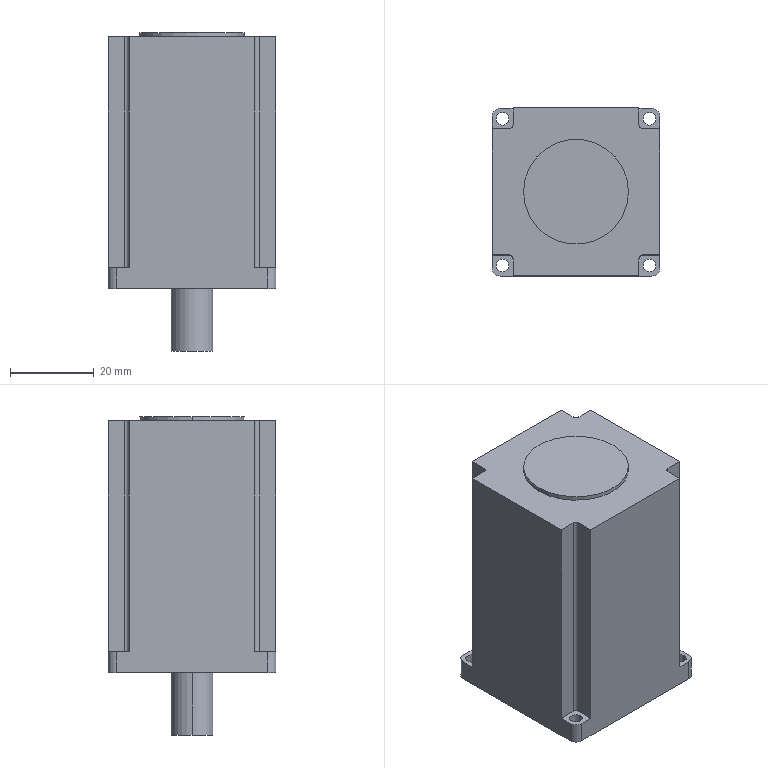Part | SolidWorks | features ICE 4, Fillet 2, Extrusion 1 | 1 solid | 40 faces | box 40 x 40 x 76 mm | volume 92058 mm3 | cylinder 20 | plane 20 | commonest cylinder face diameters 3 x8 2 x4 4 x4 10 x2 25 x2
STEP:
#1=CARTESIAN_POINT('',(-5.,0.,-45.));
#2=VERTEX_POINT('',#1);
#3=CARTESIAN_POINT('',(5.,0.,-45.));
#4=VERTEX_POINT('',#3);
#5=CARTESIAN_POINT('',(0.,0.,-45.));
#6=DIRECTION('',(0.,0.,-1.));
#7=DIRECTION('',(-1.,0.,0.));
#8=AXIS2_PLACEMENT_3D('',#5,#6,#7);
#9=CIRCLE('',#8,5.);
#10=EDGE_CURVE('',#2,#4,#9,.T.);
#11=ORIENTED_EDGE('',*,*,#10,.F.);
#12=CARTESIAN_POINT('',(-5.,0.,-30.));
#13=VERTEX_POINT('',#12);
#14=CARTESIAN_POINT('',(-5.,0.,-45.));
#15=DIRECTION('',(0.,0.,1.));
#16=VECTOR('',#15,1000.);
#17=LINE('',#14,#16);
#18=EDGE_CURVE('',#2,#13,#17,.T.);
#19=ORIENTED_EDGE('',*,*,#18,.T.);
#20=CARTESIAN_POINT('',(5.,0.,-30.));
#21=VERTEX_POINT('',#20);
#22=CARTESIAN_POINT('',(0.,0.,-30.));
#23=DIRECTION('',(0.,0.,-1.));
#24=DIRECTION('',(1.,0.,0.));
#25=AXIS2_PLACEMENT_3D('',#22,#23,#24);
#26=CIRCLE('',#25,5.);
#27=EDGE_CURVE('',#13,#21,#26,.T.);
#28=ORIENTED_EDGE('',*,*,#27,.T.);
#29=CARTESIAN_POINT('',(5.,0.,-45.));
#30=DIRECTION('',(0.,0.,1.));
#31=VECTOR('',#30,1000.);
#32=LINE('',#29,#31);
#33=EDGE_CURVE('',#4,#21,#32,.T.);
#34=ORIENTED_EDGE('',*,*,#33,.F.);
#35=EDGE_LOOP('',(#11,#19,#28,#34));
#36=FACE_OUTER_BOUND('',#35,.T.);
#37=CARTESIAN_POINT('',(0.,0.,-45.));
#38=DIRECTION('',(0.,0.,1.));
#39=DIRECTION('',(1.,0.,0.));
#40=AXIS2_PLACEMENT_3D('',#37,#38,#39);
#41=CYLINDRICAL_SURFACE('',#40,5.);
#42=ADVANCED_FACE('',(#36),#41,.T.);
#43=CARTESIAN_POINT('',(12.5,0.,31.));
#44=VERTEX_POINT('',#43);
#45=CARTESIAN_POINT('',(-12.5,0.,31.));
#46=VERTEX_POINT('',#45);
#47=CARTESIAN_POINT('',(0.,0.,31.));
#48=DIRECTION('',(0.,0.,1.));
#49=DIRECTION('',(1.,0.,0.));
#50=AXIS2_PLACEMENT_3D('',#47,#48,#49);
#51=CIRCLE('',#50,12.5);
#52=EDGE_CURVE('',#44,#46,#51,.T.);
#53=ORIENTED_EDGE('',*,*,#52,.F.);
#54=CARTESIAN_POINT('',(12.5,0.,30.));
#55=VERTEX_POINT('',#54);
#56=CARTESIAN_POINT('',(12.5,0.,31.));
#57=DIRECTION('',(0.,0.,-1.));
#58=VECTOR('',#57,1000.);
#59=LINE('',#56,#58);
#60=EDGE_CURVE('',#44,#55,#59,.T.);
#61=ORIENTED_EDGE('',*,*,#60,.T.);
#62=CARTESIAN_POINT('',(-12.5,0.,30.));
#63=VERTEX_POINT('',#62);
#64=CARTESIAN_POINT('',(0.,0.,30.));
#65=DIRECTION('',(0.,0.,-1.));
#66=DIRECTION('',(1.,0.,0.));
#67=AXIS2_PLACEMENT_3D('',#64,#65,#66);
#68=CIRCLE('',#67,12.5);
#69=EDGE_CURVE('',#63,#55,#68,.T.);
#70=ORIENTED_EDGE('',*,*,#69,.F.);
#71=CARTESIAN_POINT('',(-12.5,0.,31.));
#72=DIRECTION('',(0.,0.,-1.));
#73=VECTOR('',#72,1000.);
#74=LINE('',#71,#73);
#75=EDGE_CURVE('',#46,#63,#74,.T.);
#76=ORIENTED_EDGE('',*,*,#75,.F.);
#77=EDGE_LOOP('',(#53,#61,#70,#76));
#78=FACE_OUTER_BOUND('',#77,.T.);
#79=CARTESIAN_POINT('',(0.,0.,31.));
#80=DIRECTION('',(0.,0.,-1.));
#81=DIRECTION('',(-1.,0.,0.));
#82=AXIS2_PLACEMENT_3D('',#79,#80,#81);
#83=CYLINDRICAL_SURFACE('',#82,12.5);
#84=ADVANCED_FACE('',(#78),#83,.T.);
#85=CARTESIAN_POINT('',(-19.,17.5,-30.));
#86=VERTEX_POINT('',#85);
#87=CARTESIAN_POINT('',(-16.,17.5,-30.));
#88=VERTEX_POINT('',#87);
#89=CARTESIAN_POINT('',(-17.5,17.5,-30.));
#90=DIRECTION('',(0.,0.,1.));
#91=DIRECTION('',(1.,0.,0.));
#92=AXIS2_PLACEMENT_3D('',#89,#90,#91);
#93=CIRCLE('',#92,1.5);
#94=EDGE_CURVE('',#86,#88,#93,.T.);
#95=ORIENTED_EDGE('',*,*,#94,.F.);
#96=CARTESIAN_POINT('',(-19.,17.5,-25.));
#97=VERTEX_POINT('',#96);
#98=CARTESIAN_POINT('',(-19.,17.5,-80.));
#99=DIRECTION('',(0.,0.,1.));
#100=VECTOR('',#99,1000.);
#101=LINE('',#98,#100);
#102=EDGE_CURVE('',#86,#97,#101,.T.);
#103=ORIENTED_EDGE('',*,*,#102,.T.);
#104=CARTESIAN_POINT('',(-16.,17.5,-25.));
#105=VERTEX_POINT('',#104);
#106=CARTESIAN_POINT('',(-17.5,17.5,-25.));
#107=DIRECTION('',(0.,0.,1.));
#108=DIRECTION('',(1.,0.,0.));
#109=AXIS2_PLACEMENT_3D('',#106,#107,#108);
#110=CIRCLE('',#109,1.5);
#111=EDGE_CURVE('',#97,#105,#110,.T.);
#112=ORIENTED_EDGE('',*,*,#111,.T.);
#113=CARTESIAN_POINT('',(-16.,17.5,-80.));
#114=DIRECTION('',(0.,0.,1.));
#115=VECTOR('',#114,1000.);
#116=LINE('',#113,#115);
#117=EDGE_CURVE('',#88,#105,#116,.T.);
#118=ORIENTED_EDGE('',*,*,#117,.F.);
#119=EDGE_LOOP('',(#95,#103,#112,#118));
#120=FACE_OUTER_BOUND('',#119,.T.);
#121=CARTESIAN_POINT('',(-17.5,17.5,-80.));
#122=DIRECTION('',(0.,0.,1.));
#123=DIRECTION('',(1.,0.,0.));
#124=AXIS2_PLACEMENT_3D('',#121,#122,#123);
#125=CYLINDRICAL_SURFACE('',#124,1.5);
#126=ADVANCED_FACE('',(#120),#125,.F.);
#127=CARTESIAN_POINT('',(16.,17.5,-30.));
#128=VERTEX_POINT('',#127);
#129=CARTESIAN_POINT('',(19.,17.5,-30.));
#130=VERTEX_POINT('',#129);
#131=CARTESIAN_POINT('',(17.5,17.5,-30.));
#132=DIRECTION('',(0.,0.,1.));
#133=DIRECTION('',(1.,0.,0.));
#134=AXIS2_PLACEMENT_3D('',#131,#132,#133);
#135=CIRCLE('',#134,1.5);
#136=EDGE_CURVE('',#128,#130,#135,.T.);
#137=ORIENTED_EDGE('',*,*,#136,.F.);
#138=CARTESIAN_POINT('',(16.,17.5,-25.));
#139=VERTEX_POINT('',#138);
#140=CARTESIAN_POINT('',(16.,17.5,-80.));
#141=DIRECTION('',(0.,0.,1.));
#142=VECTOR('',#141,1000.);
#143=LINE('',#140,#142);
#144=EDGE_CURVE('',#128,#139,#143,.T.);
#145=ORIENTED_EDGE('',*,*,#144,.T.);
#146=CARTESIAN_POINT('',(19.,17.5,-25.));
#147=VERTEX_POINT('',#146);
#148=CARTESIAN_POINT('',(17.5,17.5,-25.));
#149=DIRECTION('',(0.,0.,1.));
#150=DIRECTION('',(-1.,0.,0.));
#151=AXIS2_PLACEMENT_3D('',#148,#149,#150);
#152=CIRCLE('',#151,1.5);
#153=EDGE_CURVE('',#139,#147,#152,.T.);
#154=ORIENTED_EDGE('',*,*,#153,.T.);
#155=CARTESIAN_POINT('',(19.,17.5,-80.));
#156=DIRECTION('',(0.,0.,1.));
#157=VECTOR('',#156,1000.);
#158=LINE('',#155,#157);
#159=EDGE_CURVE('',#130,#147,#158,.T.);
#160=ORIENTED_EDGE('',*,*,#159,.F.);
#161=EDGE_LOOP('',(#137,#145,#154,#160));
#162=FACE_OUTER_BOUND('',#161,.T.);
#163=CARTESIAN_POINT('',(17.5,17.5,-80.));
#164=DIRECTION('',(0.,0.,1.));
#165=DIRECTION('',(1.,0.,0.));
#166=AXIS2_PLACEMENT_3D('',#163,#164,#165);
#167=CYLINDRICAL_SURFACE('',#166,1.5);
#168=ADVANCED_FACE('',(#162),#167,.F.);
#169=CARTESIAN_POINT('',(16.,-17.5,-30.));
#170=VERTEX_POINT('',#169);
#171=CARTESIAN_POINT('',(19.,-17.5,-30.));
#172=VERTEX_POINT('',#171);
#173=CARTESIAN_POINT('',(17.5,-17.5,-30.));
#174=DIRECTION('',(0.,0.,1.));
#175=DIRECTION('',(1.,0.,0.));
#176=AXIS2_PLACEMENT_3D('',#173,#174,#175);
#177=CIRCLE('',#176,1.5);
#178=EDGE_CURVE('',#170,#172,#177,.T.);
#179=ORIENTED_EDGE('',*,*,#178,.F.);
#180=CARTESIAN_POINT('',(16.,-17.5,-25.));
#181=VERTEX_POINT('',#180);
#182=CARTESIAN_POINT('',(16.,-17.5,-80.));
#183=DIRECTION('',(0.,0.,1.));
#184=VECTOR('',#183,1000.);
#185=LINE('',#182,#184);
#186=EDGE_CURVE('',#170,#181,#185,.T.);
#187=ORIENTED_EDGE('',*,*,#186,.T.);
#188=CARTESIAN_POINT('',(19.,-17.5,-25.));
#189=VERTEX_POINT('',#188);
#190=CARTESIAN_POINT('',(17.5,-17.5,-25.));
#191=DIRECTION('',(0.,0.,1.));
#192=DIRECTION('',(1.,0.,0.));
#193=AXIS2_PLACEMENT_3D('',#190,#191,#192);
#194=CIRCLE('',#193,1.5);
#195=EDGE_CURVE('',#181,#189,#194,.T.);
#196=ORIENTED_EDGE('',*,*,#195,.T.);
#197=CARTESIAN_POINT('',(19.,-17.5,-80.));
#198=DIRECTION('',(0.,0.,1.));
#199=VECTOR('',#198,1000.);
#200=LINE('',#197,#199);
#201=EDGE_CURVE('',#172,#189,#200,.T.);
#202=ORIENTED_EDGE('',*,*,#201,.F.);
#203=EDGE_LOOP('',(#179,#187,#196,#202));
#204=FACE_OUTER_BOUND('',#203,.T.);
#205=CARTESIAN_POINT('',(17.5,-17.5,-80.));
#206=DIRECTION('',(0.,0.,1.));
#207=DIRECTION('',(1.,0.,0.));
#208=AXIS2_PLACEMENT_3D('',#205,#206,#207);
#209=CYLINDRICAL_SURFACE('',#208,1.5);
#210=ADVANCED_FACE('',(#204),#209,.F.);
#211=CARTESIAN_POINT('',(-19.,-17.5,-30.));
#212=VERTEX_POINT('',#211);
#213=CARTESIAN_POINT('',(-16.,-17.5,-30.));
#214=VERTEX_POINT('',#213);
#215=CARTESIAN_POINT('',(-17.5,-17.5,-30.));
#216=DIRECTION('',(0.,0.,1.));
#217=DIRECTION('',(1.,0.,0.));
#218=AXIS2_PLACEMENT_3D('',#215,#216,#217);
#219=CIRCLE('',#218,1.5);
#220=EDGE_CURVE('',#212,#214,#219,.T.);
#221=ORIENTED_EDGE('',*,*,#220,.F.);
#222=CARTESIAN_POINT('',(-19.,-17.5,-25.));
#223=VERTEX_POINT('',#222);
#224=CARTESIAN_POINT('',(-19.,-17.5,-80.));
#225=DIRECTION('',(0.,0.,1.));
#226=VECTOR('',#225,1000.);
#227=LINE('',#224,#226);
#228=EDGE_CURVE('',#212,#223,#227,.T.);
#229=ORIENTED_EDGE('',*,*,#228,.T.);
#230=CARTESIAN_POINT('',(-16.,-17.5,-25.));
#231=VERTEX_POINT('',#230);
#232=CARTESIAN_POINT('',(-17.5,-17.5,-25.));
#233=DIRECTION('',(0.,0.,1.));
#234=DIRECTION('',(-1.,0.,0.));
#235=AXIS2_PLACEMENT_3D('',#232,#233,#234);
#236=CIRCLE('',#235,1.5);
#237=EDGE_CURVE('',#223,#231,#236,.T.);
#238=ORIENTED_EDGE('',*,*,#237,.T.);
#239=CARTESIAN_POINT('',(-16.,-17.5,-80.));
#240=DIRECTION('',(0.,0.,1.));
#241=VECTOR('',#240,1000.);
#242=LINE('',#239,#241);
#243=EDGE_CURVE('',#214,#231,#242,.T.);
#244=ORIENTED_EDGE('',*,*,#243,.F.);
#245=EDGE_LOOP('',(#221,#229,#238,#244));
#246=FACE_OUTER_BOUND('',#245,.T.);
#247=CARTESIAN_POINT('',(-17.5,-17.5,-80.));
#248=DIRECTION('',(0.,0.,1.));
#249=DIRECTION('',(1.,0.,0.));
#250=AXIS2_PLACEMENT_3D('',#247,#248,#249);
#251=CYLINDRICAL_SURFACE('',#250,1.5);
#252=ADVANCED_FACE('',(#246),#251,.F.);
#253=CARTESIAN_POINT('',(20.,-18.,-25.));
#254=VERTEX_POINT('',#253);
#255=CARTESIAN_POINT('',(20.,-15.,-25.));
#256=VERTEX_POINT('',#255);
#257=CARTESIAN_POINT('',(20.,-20.,-25.));
#258=DIRECTION('',(0.,1.,0.));
#259=VECTOR('',#258,1000.);
#260=LINE('',#257,#259);
#261=EDGE_CURVE('',#254,#256,#260,.T.);
#262=ORIENTED_EDGE('',*,*,#261,.F.);
#263=CARTESIAN_POINT('',(20.,-18.,-30.));
#264=VERTEX_POINT('',#263);
#265=CARTESIAN_POINT('',(20.,-18.,30.));
#266=DIRECTION('',(0.,0.,-1.));
#267=VECTOR('',#266,1000.);
#268=LINE('',#265,#267);
#269=EDGE_CURVE('',#254,#264,#268,.T.);
#270=ORIENTED_EDGE('',*,*,#269,.T.);
#271=CARTESIAN_POINT('',(20.,18.,-30.));
#272=VERTEX_POINT('',#271);
#273=CARTESIAN_POINT('',(20.,20.,-30.));
#274=DIRECTION('',(0.,1.,0.));
#275=VECTOR('',#274,1000.);
#276=LINE('',#273,#275);
#277=EDGE_CURVE('',#264,#272,#276,.T.);
#278=ORIENTED_EDGE('',*,*,#277,.T.);
#279=CARTESIAN_POINT('',(20.,18.,-25.));
#280=VERTEX_POINT('',#279);
#281=CARTESIAN_POINT('',(20.,18.,30.));
#282=DIRECTION('',(0.,0.,1.));
#283=VECTOR('',#282,1000.);
#284=LINE('',#281,#283);
#285=EDGE_CURVE('',#272,#280,#284,.T.);
#286=ORIENTED_EDGE('',*,*,#285,.T.);
#287=CARTESIAN_POINT('',(20.,15.,-25.));
#288=VERTEX_POINT('',#287);
#289=CARTESIAN_POINT('',(20.,20.,-25.));
#290=DIRECTION('',(0.,1.,0.));
#291=VECTOR('',#290,1000.);
#292=LINE('',#289,#291);
#293=EDGE_CURVE('',#288,#280,#292,.T.);
#294=ORIENTED_EDGE('',*,*,#293,.F.);
#295=CARTESIAN_POINT('',(20.,15.,30.));
#296=VERTEX_POINT('',#295);
#297=CARTESIAN_POINT('',(20.,15.,-25.));
#298=DIRECTION('',(0.,0.,1.));
#299=VECTOR('',#298,1000.);
#300=LINE('',#297,#299);
#301=EDGE_CURVE('',#288,#296,#300,.T.);
#302=ORIENTED_EDGE('',*,*,#301,.T.);
#303=CARTESIAN_POINT('',(20.,-15.,30.));
#304=VERTEX_POINT('',#303);
#305=CARTESIAN_POINT('',(20.,20.,30.));
#306=DIRECTION('',(0.,1.,0.));
#307=VECTOR('',#306,1000.);
#308=LINE('',#305,#307);
#309=EDGE_CURVE('',#304,#296,#308,.T.);
#310=ORIENTED_EDGE('',*,*,#309,.F.);
#311=CARTESIAN_POINT('',(20.,-15.,-25.));
#312=DIRECTION('',(0.,0.,1.));
#313=VECTOR('',#312,1000.);
#314=LINE('',#311,#313);
#315=EDGE_CURVE('',#256,#304,#314,.T.);
#316=ORIENTED_EDGE('',*,*,#315,.F.);
#317=EDGE_LOOP('',(#262,#270,#278,#286,#294,#302,#310,#316));
#318=FACE_OUTER_BOUND('',#317,.T.);
#319=CARTESIAN_POINT('',(20.,20.,30.));
#320=DIRECTION('',(-1.,0.,0.));
#321=DIRECTION('',(0.,-1.,0.));
#322=AXIS2_PLACEMENT_3D('',#319,#320,#321);
#323=PLANE('',#322);
#324=ADVANCED_FACE('',(#318),#323,.F.);
#325=CARTESIAN_POINT('',(18.,20.,-25.));
#326=VERTEX_POINT('',#325);
#327=CARTESIAN_POINT('',(15.,20.,-25.));
#328=VERTEX_POINT('',#327);
#329=CARTESIAN_POINT('',(20.,20.,-25.));
#330=DIRECTION('',(-1.,0.,0.));
#331=VECTOR('',#330,1000.);
#332=LINE('',#329,#331);
#333=EDGE_CURVE('',#326,#328,#332,.T.);
#334=ORIENTED_EDGE('',*,*,#333,.F.);
#335=CARTESIAN_POINT('',(18.,20.,-30.));
#336=VERTEX_POINT('',#335);
#337=CARTESIAN_POINT('',(18.,20.,30.));
#338=DIRECTION('',(0.,0.,-1.));
#339=VECTOR('',#338,1000.);
#340=LINE('',#337,#339);
#341=EDGE_CURVE('',#326,#336,#340,.T.);
#342=ORIENTED_EDGE('',*,*,#341,.T.);
#343=CARTESIAN_POINT('',(-18.,20.,-30.));
#344=VERTEX_POINT('',#343);
#345=CARTESIAN_POINT('',(-20.,20.,-30.));
#346=DIRECTION('',(-1.,0.,0.));
#347=VECTOR('',#346,1000.);
#348=LINE('',#345,#347);
#349=EDGE_CURVE('',#336,#344,#348,.T.);
#350=ORIENTED_EDGE('',*,*,#349,.T.);
#351=CARTESIAN_POINT('',(-18.,20.,-25.));
#352=VERTEX_POINT('',#351);
#353=CARTESIAN_POINT('',(-18.,20.,30.));
#354=DIRECTION('',(0.,0.,1.));
#355=VECTOR('',#354,1000.);
#356=LINE('',#353,#355);
#357=EDGE_CURVE('',#344,#352,#356,.T.);
#358=ORIENTED_EDGE('',*,*,#357,.T.);
#359=CARTESIAN_POINT('',(-15.,20.,-25.));
#360=VERTEX_POINT('',#359);
#361=CARTESIAN_POINT('',(-20.,20.,-25.));
#362=DIRECTION('',(-1.,0.,0.));
#363=VECTOR('',#362,1000.);
#364=LINE('',#361,#363);
#365=EDGE_CURVE('',#360,#352,#364,.T.);
#366=ORIENTED_EDGE('',*,*,#365,.F.);
#367=CARTESIAN_POINT('',(-15.,20.,30.));
#368=VERTEX_POINT('',#367);
#369=CARTESIAN_POINT('',(-15.,20.,-25.));
#370=DIRECTION('',(0.,0.,1.));
#371=VECTOR('',#370,1000.);
#372=LINE('',#369,#371);
#373=EDGE_CURVE('',#360,#368,#372,.T.);
#374=ORIENTED_EDGE('',*,*,#373,.T.);
#375=CARTESIAN_POINT('',(15.,20.,30.));
#376=VERTEX_POINT('',#375);
#377=CARTESIAN_POINT('',(-20.,20.,30.));
#378=DIRECTION('',(-1.,0.,0.));
#379=VECTOR('',#378,1000.);
#380=LINE('',#377,#379);
#381=EDGE_CURVE('',#376,#368,#380,.T.);
#382=ORIENTED_EDGE('',*,*,#381,.F.);
#383=CARTESIAN_POINT('',(15.,20.,-25.));
#384=DIRECTION('',(0.,0.,1.));
#385=VECTOR('',#384,1000.);
#386=LINE('',#383,#385);
#387=EDGE_CURVE('',#328,#376,#386,.T.);
#388=ORIENTED_EDGE('',*,*,#387,.F.);
#389=EDGE_LOOP('',(#334,#342,#350,#358,#366,#374,#382,#388));
#390=FACE_OUTER_BOUND('',#389,.T.);
#391=CARTESIAN_POINT('',(-20.,20.,30.));
#392=DIRECTION('',(0.,-1.,0.));
#393=DIRECTION('',(0.,0.,-1.));
#394=AXIS2_PLACEMENT_3D('',#391,#392,#393);
#395=PLANE('',#394);
#396=ADVANCED_FACE('',(#390),#395,.F.);
#397=CARTESIAN_POINT('',(-20.,18.,-30.));
#398=VERTEX_POINT('',#397);
#399=CARTESIAN_POINT('',(-20.,-18.,-30.));
#400=VERTEX_POINT('',#399);
#401=CARTESIAN_POINT('',(-20.,20.,-30.));
#402=DIRECTION('',(0.,-1.,0.));
#403=VECTOR('',#402,1000.);
#404=LINE('',#401,#403);
#405=EDGE_CURVE('',#398,#400,#404,.T.);
#406=ORIENTED_EDGE('',*,*,#405,.T.);
#407=CARTESIAN_POINT('',(-20.,-18.,-25.));
#408=VERTEX_POINT('',#407);
#409=CARTESIAN_POINT('',(-20.,-18.,30.));
#410=DIRECTION('',(0.,0.,1.));
#411=VECTOR('',#410,1000.);
#412=LINE('',#409,#411);
#413=EDGE_CURVE('',#400,#408,#412,.T.);
#414=ORIENTED_EDGE('',*,*,#413,.T.);
#415=CARTESIAN_POINT('',(-20.,-15.,-25.));
#416=VERTEX_POINT('',#415);
#417=CARTESIAN_POINT('',(-20.,-20.,-25.));
#418=DIRECTION('',(0.,-1.,0.));
#419=VECTOR('',#418,1000.);
#420=LINE('',#417,#419);
#421=EDGE_CURVE('',#416,#408,#420,.T.);
#422=ORIENTED_EDGE('',*,*,#421,.F.);
#423=CARTESIAN_POINT('',(-20.,-15.,30.));
#424=VERTEX_POINT('',#423);
#425=CARTESIAN_POINT('',(-20.,-15.,-25.));
#426=DIRECTION('',(0.,0.,1.));
#427=VECTOR('',#426,1000.);
#428=LINE('',#425,#427);
#429=EDGE_CURVE('',#416,#424,#428,.T.);
#430=ORIENTED_EDGE('',*,*,#429,.T.);
#431=CARTESIAN_POINT('',(-20.,15.,30.));
#432=VERTEX_POINT('',#431);
#433=CARTESIAN_POINT('',(-20.,20.,30.));
#434=DIRECTION('',(0.,-1.,0.));
#435=VECTOR('',#434,1000.);
#436=LINE('',#433,#435);
#437=EDGE_CURVE('',#432,#424,#436,.T.);
#438=ORIENTED_EDGE('',*,*,#437,.F.);
#439=CARTESIAN_POINT('',(-20.,15.,-25.));
#440=VERTEX_POINT('',#439);
#441=CARTESIAN_POINT('',(-20.,15.,-25.));
#442=DIRECTION('',(0.,0.,1.));
#443=VECTOR('',#442,1000.);
#444=LINE('',#441,#443);
#445=EDGE_CURVE('',#440,#432,#444,.T.);
#446=ORIENTED_EDGE('',*,*,#445,.F.);
#447=CARTESIAN_POINT('',(-20.,18.,-25.));
#448=VERTEX_POINT('',#447);
#449=CARTESIAN_POINT('',(-20.,20.,-25.));
#450=DIRECTION('',(0.,-1.,0.));
#451=VECTOR('',#450,1000.);
#452=LINE('',#449,#451);
#453=EDGE_CURVE('',#448,#440,#452,.T.);
#454=ORIENTED_EDGE('',*,*,#453,.F.);
#455=CARTESIAN_POINT('',(-20.,18.,30.));
#456=DIRECTION('',(0.,0.,-1.));
#457=VECTOR('',#456,1000.);
#458=LINE('',#455,#457);
#459=EDGE_CURVE('',#448,#398,#458,.T.);
#460=ORIENTED_EDGE('',*,*,#459,.T.);
#461=EDGE_LOOP('',(#406,#414,#422,#430,#438,#446,#454,#460));
#462=FACE_OUTER_BOUND('',#461,.T.);
#463=CARTESIAN_POINT('',(-20.,20.,30.));
#464=DIRECTION('',(1.,0.,0.));
#465=DIRECTION('',(0.,1.,0.));
#466=AXIS2_PLACEMENT_3D('',#463,#464,#465);
#467=PLANE('',#466);
#468=ADVANCED_FACE('',(#462),#467,.F.);
#469=CARTESIAN_POINT('',(-18.,-20.,-25.));
#470=VERTEX_POINT('',#469);
#471=CARTESIAN_POINT('',(-15.,-20.,-25.));
#472=VERTEX_POINT('',#471);
#473=CARTESIAN_POINT('',(-20.,-20.,-25.));
#474=DIRECTION('',(1.,0.,0.));
#475=VECTOR('',#474,1000.);
#476=LINE('',#473,#475);
#477=EDGE_CURVE('',#470,#472,#476,.T.);
#478=ORIENTED_EDGE('',*,*,#477,.F.);
#479=CARTESIAN_POINT('',(-18.,-20.,-30.));
#480=VERTEX_POINT('',#479);
#481=CARTESIAN_POINT('',(-18.,-20.,30.));
#482=DIRECTION('',(0.,0.,-1.));
#483=VECTOR('',#482,1000.);
#484=LINE('',#481,#483);
#485=EDGE_CURVE('',#470,#480,#484,.T.);
#486=ORIENTED_EDGE('',*,*,#485,.T.);
#487=CARTESIAN_POINT('',(18.,-20.,-30.));
#488=VERTEX_POINT('',#487);
#489=CARTESIAN_POINT('',(-20.,-20.,-30.));
#490=DIRECTION('',(1.,0.,0.));
#491=VECTOR('',#490,1000.);
#492=LINE('',#489,#491);
#493=EDGE_CURVE('',#480,#488,#492,.T.);
#494=ORIENTED_EDGE('',*,*,#493,.T.);
#495=CARTESIAN_POINT('',(18.,-20.,-25.));
#496=VERTEX_POINT('',#495);
#497=CARTESIAN_POINT('',(18.,-20.,30.));
#498=DIRECTION('',(0.,0.,1.));
#499=VECTOR('',#498,1000.);
#500=LINE('',#497,#499);
#501=EDGE_CURVE('',#488,#496,#500,.T.);
#502=ORIENTED_EDGE('',*,*,#501,.T.);
#503=CARTESIAN_POINT('',(15.,-20.,-25.));
#504=VERTEX_POINT('',#503);
#505=CARTESIAN_POINT('',(20.,-20.,-25.));
#506=DIRECTION('',(1.,0.,0.));
#507=VECTOR('',#506,1000.);
#508=LINE('',#505,#507);
#509=EDGE_CURVE('',#504,#496,#508,.T.);
#510=ORIENTED_EDGE('',*,*,#509,.F.);
#511=CARTESIAN_POINT('',(15.,-20.,30.));
#512=VERTEX_POINT('',#511);
#513=CARTESIAN_POINT('',(15.,-20.,-25.));
#514=DIRECTION('',(0.,0.,1.));
#515=VECTOR('',#514,1000.);
#516=LINE('',#513,#515);
#517=EDGE_CURVE('',#504,#512,#516,.T.);
#518=ORIENTED_EDGE('',*,*,#517,.T.);
#519=CARTESIAN_POINT('',(-15.,-20.,30.));
#520=VERTEX_POINT('',#519);
#521=CARTESIAN_POINT('',(-20.,-20.,30.));
#522=DIRECTION('',(1.,0.,0.));
#523=VECTOR('',#522,1000.);
#524=LINE('',#521,#523);
#525=EDGE_CURVE('',#520,#512,#524,.T.);
#526=ORIENTED_EDGE('',*,*,#525,.F.);
#527=CARTESIAN_POINT('',(-15.,-20.,-25.));
#528=DIRECTION('',(0.,0.,1.));
#529=VECTOR('',#528,1000.);
#530=LINE('',#527,#529);
#531=EDGE_CURVE('',#472,#520,#530,.T.);
#532=ORIENTED_EDGE('',*,*,#531,.F.);
#533=EDGE_LOOP('',(#478,#486,#494,#502,#510,#518,#526,#532));
#534=FACE_OUTER_BOUND('',#533,.T.);
#535=CARTESIAN_POINT('',(-20.,-20.,30.));
#536=DIRECTION('',(0.,1.,0.));
#537=DIRECTION('',(0.,0.,1.));
#538=AXIS2_PLACEMENT_3D('',#535,#536,#537);
#539=PLANE('',#538);
#540=ADVANCED_FACE('',(#534),#539,.F.);
#541=ORIENTED_EDGE('',*,*,#69,.T.);
#542=CARTESIAN_POINT('',(0.,0.,30.));
#543=DIRECTION('',(0.,0.,-1.));
#544=DIRECTION('',(1.,0.,0.));
#545=AXIS2_PLACEMENT_3D('',#542,#543,#544);
#546=CIRCLE('',#545,12.5);
#547=EDGE_CURVE('',#55,#63,#546,.T.);
#548=ORIENTED_EDGE('',*,*,#547,.T.);
#549=EDGE_LOOP('',(#541,#548));
#550=FACE_BOUND('',#549,.T.);
#551=CARTESIAN_POINT('',(-16.,-15.,30.));
#552=VERTEX_POINT('',#551);
#553=CARTESIAN_POINT('',(-20.,-15.,30.));
#554=DIRECTION('',(-1.,0.,0.));
#555=VECTOR('',#554,1000.);
#556=LINE('',#553,#555);
#557=EDGE_CURVE('',#552,#424,#556,.T.);
#558=ORIENTED_EDGE('',*,*,#557,.F.);
#559=CARTESIAN_POINT('',(-15.,-16.,30.));
#560=VERTEX_POINT('',#559);
#561=CARTESIAN_POINT('',(-16.,-16.,30.));
#562=DIRECTION('',(0.,0.,-1.));
#563=DIRECTION('',(1.,0.,0.));
#564=AXIS2_PLACEMENT_3D('',#561,#562,#563);
#565=CIRCLE('',#564,1.);
#566=EDGE_CURVE('',#552,#560,#565,.T.);
#567=ORIENTED_EDGE('',*,*,#566,.T.);
#568=CARTESIAN_POINT('',(-15.,-20.,30.));
#569=DIRECTION('',(0.,1.,0.));
#570=VECTOR('',#569,1000.);
#571=LINE('',#568,#570);
#572=EDGE_CURVE('',#520,#560,#571,.T.);
#573=ORIENTED_EDGE('',*,*,#572,.F.);
#574=ORIENTED_EDGE('',*,*,#525,.T.);
#575=CARTESIAN_POINT('',(15.,-16.,30.));
#576=VERTEX_POINT('',#575);
#577=CARTESIAN_POINT('',(15.,-20.,30.));
#578=DIRECTION('',(0.,-1.,0.));
#579=VECTOR('',#578,1000.);
#580=LINE('',#577,#579);
#581=EDGE_CURVE('',#576,#512,#580,.T.);
#582=ORIENTED_EDGE('',*,*,#581,.F.);
#583=CARTESIAN_POINT('',(16.,-15.,30.));
#584=VERTEX_POINT('',#583);
#585=CARTESIAN_POINT('',(16.,-16.,30.));
#586=DIRECTION('',(0.,0.,-1.));
#587=DIRECTION('',(1.,0.,0.));
#588=AXIS2_PLACEMENT_3D('',#585,#586,#587);
#589=CIRCLE('',#588,1.);
#590=EDGE_CURVE('',#576,#584,#589,.T.);
#591=ORIENTED_EDGE('',*,*,#590,.T.);
#592=CARTESIAN_POINT('',(20.,-15.,30.));
#593=DIRECTION('',(-1.,0.,0.));
#594=VECTOR('',#593,1000.);
#595=LINE('',#592,#594);
#596=EDGE_CURVE('',#304,#584,#595,.T.);
#597=ORIENTED_EDGE('',*,*,#596,.F.);
#598=ORIENTED_EDGE('',*,*,#309,.T.);
#599=CARTESIAN_POINT('',(16.,15.,30.));
#600=VERTEX_POINT('',#599);
#601=CARTESIAN_POINT('',(20.,15.,30.));
#602=DIRECTION('',(1.,0.,0.));
#603=VECTOR('',#602,1000.);
#604=LINE('',#601,#603);
#605=EDGE_CURVE('',#600,#296,#604,.T.);
#606=ORIENTED_EDGE('',*,*,#605,.F.);
#607=CARTESIAN_POINT('',(15.,16.,30.));
#608=VERTEX_POINT('',#607);
#609=CARTESIAN_POINT('',(16.,16.,30.));
#610=DIRECTION('',(0.,0.,-1.));
#611=DIRECTION('',(1.,0.,0.));
#612=AXIS2_PLACEMENT_3D('',#609,#610,#611);
#613=CIRCLE('',#612,1.);
#614=EDGE_CURVE('',#600,#608,#613,.T.);
#615=ORIENTED_EDGE('',*,*,#614,.T.);
#616=CARTESIAN_POINT('',(15.,20.,30.));
#617=DIRECTION('',(0.,-1.,0.));
#618=VECTOR('',#617,1000.);
#619=LINE('',#616,#618);
#620=EDGE_CURVE('',#376,#608,#619,.T.);
#621=ORIENTED_EDGE('',*,*,#620,.F.);
#622=ORIENTED_EDGE('',*,*,#381,.T.);
#623=CARTESIAN_POINT('',(-15.,16.,30.));
#624=VERTEX_POINT('',#623);
#625=CARTESIAN_POINT('',(-15.,20.,30.));
#626=DIRECTION('',(0.,1.,0.));
#627=VECTOR('',#626,1000.);
#628=LINE('',#625,#627);
#629=EDGE_CURVE('',#624,#368,#628,.T.);
#630=ORIENTED_EDGE('',*,*,#629,.F.);
#631=CARTESIAN_POINT('',(-16.,15.,30.));
#632=VERTEX_POINT('',#631);
#633=CARTESIAN_POINT('',(-16.,16.,30.));
#634=DIRECTION('',(0.,0.,-1.));
#635=DIRECTION('',(1.,0.,0.));
#636=AXIS2_PLACEMENT_3D('',#633,#634,#635);
#637=CIRCLE('',#636,1.);
#638=EDGE_CURVE('',#624,#632,#637,.T.);
#639=ORIENTED_EDGE('',*,*,#638,.T.);
#640=CARTESIAN_POINT('',(-20.,15.,30.));
#641=DIRECTION('',(1.,0.,0.));
#642=VECTOR('',#641,1000.);
#643=LINE('',#640,#642);
#644=EDGE_CURVE('',#432,#632,#643,.T.);
#645=ORIENTED_EDGE('',*,*,#644,.F.);
#646=ORIENTED_EDGE('',*,*,#437,.T.);
#647=EDGE_LOOP('',(#558,#567,#573,#574,#582,#591,#597,#598,#606,#615,#621,#622,#630,#639,#645,#646));
#648=FACE_OUTER_BOUND('',#647,.T.);
#649=CARTESIAN_POINT('',(0.,0.,30.));
#650=DIRECTION('',(0.,0.,1.));
#651=DIRECTION('',(1.,0.,0.));
#652=AXIS2_PLACEMENT_3D('',#649,#650,#651);
#653=PLANE('',#652);
#654=ADVANCED_FACE('',(#550,#648),#653,.T.);
#655=CARTESIAN_POINT('',(0.,0.,-30.));
#656=DIRECTION('',(0.,0.,-1.));
#657=DIRECTION('',(1.,0.,0.));
#658=AXIS2_PLACEMENT_3D('',#655,#656,#657);
#659=CIRCLE('',#658,5.);
#660=EDGE_CURVE('',#21,#13,#659,.T.);
#661=ORIENTED_EDGE('',*,*,#660,.F.);
#662=ORIENTED_EDGE('',*,*,#27,.F.);
#663=EDGE_LOOP('',(#661,#662));
#664=FACE_BOUND('',#663,.T.);
#665=CARTESIAN_POINT('',(-17.5,-17.5,-30.));
#666=DIRECTION('',(0.,0.,1.));
#667=DIRECTION('',(1.,0.,0.));
#668=AXIS2_PLACEMENT_3D('',#665,#666,#667);
#669=CIRCLE('',#668,1.5);
#670=EDGE_CURVE('',#214,#212,#669,.T.);
#671=ORIENTED_EDGE('',*,*,#670,.T.);
#672=ORIENTED_EDGE('',*,*,#220,.T.);
#673=EDGE_LOOP('',(#671,#672));
#674=FACE_BOUND('',#673,.T.);
#675=CARTESIAN_POINT('',(17.5,-17.5,-30.));
#676=DIRECTION('',(0.,0.,1.));
#677=DIRECTION('',(1.,0.,0.));
#678=AXIS2_PLACEMENT_3D('',#675,#676,#677);
#679=CIRCLE('',#678,1.5);
#680=EDGE_CURVE('',#172,#170,#679,.T.);
#681=ORIENTED_EDGE('',*,*,#680,.T.);
#682=ORIENTED_EDGE('',*,*,#178,.T.);
#683=EDGE_LOOP('',(#681,#682));
#684=FACE_BOUND('',#683,.T.);
#685=CARTESIAN_POINT('',(17.5,17.5,-30.));
#686=DIRECTION('',(0.,0.,1.));
#687=DIRECTION('',(1.,0.,0.));
#688=AXIS2_PLACEMENT_3D('',#685,#686,#687);
#689=CIRCLE('',#688,1.5);
#690=EDGE_CURVE('',#130,#128,#689,.T.);
#691=ORIENTED_EDGE('',*,*,#690,.T.);
#692=ORIENTED_EDGE('',*,*,#136,.T.);
#693=EDGE_LOOP('',(#691,#692));
#694=FACE_BOUND('',#693,.T.);
#695=CARTESIAN_POINT('',(-17.5,17.5,-30.));
#696=DIRECTION('',(0.,0.,1.));
#697=DIRECTION('',(1.,0.,0.));
#698=AXIS2_PLACEMENT_3D('',#695,#696,#697);
#699=CIRCLE('',#698,1.5);
#700=EDGE_CURVE('',#88,#86,#699,.T.);
#701=ORIENTED_EDGE('',*,*,#700,.T.);
#702=ORIENTED_EDGE('',*,*,#94,.T.);
#703=EDGE_LOOP('',(#701,#702));
#704=FACE_BOUND('',#703,.T.);
#705=ORIENTED_EDGE('',*,*,#493,.F.);
#706=CARTESIAN_POINT('',(-18.,-18.,-30.));
#707=DIRECTION('',(0.,0.,-1.));
#708=DIRECTION('',(1.,0.,0.));
#709=AXIS2_PLACEMENT_3D('',#706,#707,#708);
#710=CIRCLE('',#709,2.);
#711=EDGE_CURVE('',#480,#400,#710,.T.);
#712=ORIENTED_EDGE('',*,*,#711,.T.);
#713=ORIENTED_EDGE('',*,*,#405,.F.);
#714=CARTESIAN_POINT('',(-18.,18.,-30.));
#715=DIRECTION('',(0.,0.,-1.));
#716=DIRECTION('',(1.,0.,0.));
#717=AXIS2_PLACEMENT_3D('',#714,#715,#716);
#718=CIRCLE('',#717,2.);
#719=EDGE_CURVE('',#398,#344,#718,.T.);
#720=ORIENTED_EDGE('',*,*,#719,.T.);
#721=ORIENTED_EDGE('',*,*,#349,.F.);
#722=CARTESIAN_POINT('',(18.,18.,-30.));
#723=DIRECTION('',(0.,0.,-1.));
#724=DIRECTION('',(1.,0.,0.));
#725=AXIS2_PLACEMENT_3D('',#722,#723,#724);
#726=CIRCLE('',#725,2.);
#727=EDGE_CURVE('',#336,#272,#726,.T.);
#728=ORIENTED_EDGE('',*,*,#727,.T.);
#729=ORIENTED_EDGE('',*,*,#277,.F.);
#730=CARTESIAN_POINT('',(18.,-18.,-30.));
#731=DIRECTION('',(0.,0.,-1.));
#732=DIRECTION('',(1.,0.,0.));
#733=AXIS2_PLACEMENT_3D('',#730,#731,#732);
#734=CIRCLE('',#733,2.);
#735=EDGE_CURVE('',#264,#488,#734,.T.);
#736=ORIENTED_EDGE('',*,*,#735,.T.);
#737=EDGE_LOOP('',(#705,#712,#713,#720,#721,#728,#729,#736));
#738=FACE_OUTER_BOUND('',#737,.T.);
#739=CARTESIAN_POINT('',(0.,0.,-30.));
#740=DIRECTION('',(0.,0.,1.));
#741=DIRECTION('',(1.,0.,0.));
#742=AXIS2_PLACEMENT_3D('',#739,#740,#741);
#743=PLANE('',#742);
#744=ADVANCED_FACE('',(#664,#674,#684,#694,#704,#738),#743,.F.);
#745=CARTESIAN_POINT('',(-15.,16.,-25.));
#746=VERTEX_POINT('',#745);
#747=CARTESIAN_POINT('',(-15.,20.,-25.));
#748=DIRECTION('',(0.,1.,0.));
#749=VECTOR('',#748,1000.);
#750=LINE('',#747,#749);
#751=EDGE_CURVE('',#746,#360,#750,.T.);
#752=ORIENTED_EDGE('',*,*,#751,.F.);
#753=CARTESIAN_POINT('',(-15.,16.,30.));
#754=DIRECTION('',(0.,0.,1.));
#755=VECTOR('',#754,1000.);
#756=LINE('',#753,#755);
#757=EDGE_CURVE('',#746,#624,#756,.T.);
#758=ORIENTED_EDGE('',*,*,#757,.T.);
#759=ORIENTED_EDGE('',*,*,#629,.T.);
#760=ORIENTED_EDGE('',*,*,#373,.F.);
#761=EDGE_LOOP('',(#752,#758,#759,#760));
#762=FACE_OUTER_BOUND('',#761,.T.);
#763=CARTESIAN_POINT('',(-15.,20.,-25.));
#764=DIRECTION('',(1.,0.,0.));
#765=DIRECTION('',(0.,0.,-1.));
#766=AXIS2_PLACEMENT_3D('',#763,#764,#765);
#767=PLANE('',#766);
#768=ADVANCED_FACE('',(#762),#767,.F.);
#769=ORIENTED_EDGE('',*,*,#644,.T.);
#770=CARTESIAN_POINT('',(-16.,15.,-25.));
#771=VERTEX_POINT('',#770);
#772=CARTESIAN_POINT('',(-16.,15.,-25.));
#773=DIRECTION('',(0.,0.,-1.));
#774=VECTOR('',#773,1000.);
#775=LINE('',#772,#774);
#776=EDGE_CURVE('',#632,#771,#775,.T.);
#777=ORIENTED_EDGE('',*,*,#776,.T.);
#778=CARTESIAN_POINT('',(-20.,15.,-25.));
#779=DIRECTION('',(1.,0.,0.));
#780=VECTOR('',#779,1000.);
#781=LINE('',#778,#780);
#782=EDGE_CURVE('',#440,#771,#781,.T.);
#783=ORIENTED_EDGE('',*,*,#782,.F.);
#784=ORIENTED_EDGE('',*,*,#445,.T.);
#785=EDGE_LOOP('',(#769,#777,#783,#784));
#786=FACE_OUTER_BOUND('',#785,.T.);
#787=CARTESIAN_POINT('',(-20.,15.,-25.));
#788=DIRECTION('',(0.,-1.,0.));
#789=DIRECTION('',(1.,0.,0.));
#790=AXIS2_PLACEMENT_3D('',#787,#788,#789);
#791=PLANE('',#790);
#792=ADVANCED_FACE('',(#786),#791,.F.);
#793=CARTESIAN_POINT('',(-17.5,17.5,-25.));
#794=DIRECTION('',(0.,0.,1.));
#795=DIRECTION('',(1.,0.,0.));
#796=AXIS2_PLACEMENT_3D('',#793,#794,#795);
#797=CIRCLE('',#796,1.5);
#798=EDGE_CURVE('',#105,#97,#797,.T.);
#799=ORIENTED_EDGE('',*,*,#798,.F.);
#800=ORIENTED_EDGE('',*,*,#111,.F.);
#801=EDGE_LOOP('',(#799,#800));
#802=FACE_BOUND('',#801,.T.);
#803=ORIENTED_EDGE('',*,*,#782,.T.);
#804=CARTESIAN_POINT('',(-16.,16.,-25.));
#805=DIRECTION('',(0.,0.,1.));
#806=DIRECTION('',(1.,0.,0.));
#807=AXIS2_PLACEMENT_3D('',#804,#805,#806);
#808=CIRCLE('',#807,1.);
#809=EDGE_CURVE('',#771,#746,#808,.T.);
#810=ORIENTED_EDGE('',*,*,#809,.T.);
#811=ORIENTED_EDGE('',*,*,#751,.T.);
#812=ORIENTED_EDGE('',*,*,#365,.T.);
#813=CARTESIAN_POINT('',(-18.,18.,-25.));
#814=DIRECTION('',(0.,0.,1.));
#815=DIRECTION('',(1.,0.,0.));
#816=AXIS2_PLACEMENT_3D('',#813,#814,#815);
#817=CIRCLE('',#816,2.);
#818=EDGE_CURVE('',#352,#448,#817,.T.);
#819=ORIENTED_EDGE('',*,*,#818,.T.);
#820=ORIENTED_EDGE('',*,*,#453,.T.);
#821=EDGE_LOOP('',(#803,#810,#811,#812,#819,#820));
#822=FACE_OUTER_BOUND('',#821,.T.);
#823=CARTESIAN_POINT('',(0.,0.,-25.));
#824=DIRECTION('',(0.,0.,1.));
#825=DIRECTION('',(1.,0.,0.));
#826=AXIS2_PLACEMENT_3D('',#823,#824,#825);
#827=PLANE('',#826);
#828=ADVANCED_FACE('',(#802,#822),#827,.T.);
#829=CARTESIAN_POINT('',(16.,15.,-25.));
#830=VERTEX_POINT('',#829);
#831=CARTESIAN_POINT('',(20.,15.,-25.));
#832=DIRECTION('',(1.,0.,0.));
#833=VECTOR('',#832,1000.);
#834=LINE('',#831,#833);
#835=EDGE_CURVE('',#830,#288,#834,.T.);
#836=ORIENTED_EDGE('',*,*,#835,.F.);
#837=CARTESIAN_POINT('',(16.,15.,30.));
#838=DIRECTION('',(0.,0.,1.));
#839=VECTOR('',#838,1000.);
#840=LINE('',#837,#839);
#841=EDGE_CURVE('',#830,#600,#840,.T.);
#842=ORIENTED_EDGE('',*,*,#841,.T.);
#843=ORIENTED_EDGE('',*,*,#605,.T.);
#844=ORIENTED_EDGE('',*,*,#301,.F.);
#845=EDGE_LOOP('',(#836,#842,#843,#844));
#846=FACE_OUTER_BOUND('',#845,.T.);
#847=CARTESIAN_POINT('',(20.,15.,-25.));
#848=DIRECTION('',(0.,-1.,0.));
#849=DIRECTION('',(1.,0.,0.));
#850=AXIS2_PLACEMENT_3D('',#847,#848,#849);
#851=PLANE('',#850);
#852=ADVANCED_FACE('',(#846),#851,.F.);
#853=ORIENTED_EDGE('',*,*,#620,.T.);
#854=CARTESIAN_POINT('',(15.,16.,-25.));
#855=VERTEX_POINT('',#854);
#856=CARTESIAN_POINT('',(15.,16.,-25.));
#857=DIRECTION('',(0.,0.,-1.));
#858=VECTOR('',#857,1000.);
#859=LINE('',#856,#858);
#860=EDGE_CURVE('',#608,#855,#859,.T.);
#861=ORIENTED_EDGE('',*,*,#860,.T.);
#862=CARTESIAN_POINT('',(15.,20.,-25.));
#863=DIRECTION('',(0.,-1.,0.));
#864=VECTOR('',#863,1000.);
#865=LINE('',#862,#864);
#866=EDGE_CURVE('',#328,#855,#865,.T.);
#867=ORIENTED_EDGE('',*,*,#866,.F.);
#868=ORIENTED_EDGE('',*,*,#387,.T.);
#869=EDGE_LOOP('',(#853,#861,#867,#868));
#870=FACE_OUTER_BOUND('',#869,.T.);
#871=CARTESIAN_POINT('',(15.,20.,-25.));
#872=DIRECTION('',(-1.,0.,0.));
#873=DIRECTION('',(0.,0.,1.));
#874=AXIS2_PLACEMENT_3D('',#871,#872,#873);
#875=PLANE('',#874);
#876=ADVANCED_FACE('',(#870),#875,.F.);
#877=CARTESIAN_POINT('',(17.5,17.5,-25.));
#878=DIRECTION('',(0.,0.,1.));
#879=DIRECTION('',(-1.,0.,0.));
#880=AXIS2_PLACEMENT_3D('',#877,#878,#879);
#881=CIRCLE('',#880,1.5);
#882=EDGE_CURVE('',#147,#139,#881,.T.);
#883=ORIENTED_EDGE('',*,*,#882,.F.);
#884=ORIENTED_EDGE('',*,*,#153,.F.);
#885=EDGE_LOOP('',(#883,#884));
#886=FACE_BOUND('',#885,.T.);
#887=ORIENTED_EDGE('',*,*,#866,.T.);
#888=CARTESIAN_POINT('',(16.,16.,-25.));
#889=DIRECTION('',(0.,0.,1.));
#890=DIRECTION('',(-1.,0.,0.));
#891=AXIS2_PLACEMENT_3D('',#888,#889,#890);
#892=CIRCLE('',#891,1.);
#893=EDGE_CURVE('',#855,#830,#892,.T.);
#894=ORIENTED_EDGE('',*,*,#893,.T.);
#895=ORIENTED_EDGE('',*,*,#835,.T.);
#896=ORIENTED_EDGE('',*,*,#293,.T.);
#897=CARTESIAN_POINT('',(18.,18.,-25.));
#898=DIRECTION('',(0.,0.,1.));
#899=DIRECTION('',(-1.,0.,0.));
#900=AXIS2_PLACEMENT_3D('',#897,#898,#899);
#901=CIRCLE('',#900,2.);
#902=EDGE_CURVE('',#280,#326,#901,.T.);
#903=ORIENTED_EDGE('',*,*,#902,.T.);
#904=ORIENTED_EDGE('',*,*,#333,.T.);
#905=EDGE_LOOP('',(#887,#894,#895,#896,#903,#904));
#906=FACE_OUTER_BOUND('',#905,.T.);
#907=CARTESIAN_POINT('',(0.,0.,-25.));
#908=DIRECTION('',(0.,0.,-1.));
#909=DIRECTION('',(-1.,0.,0.));
#910=AXIS2_PLACEMENT_3D('',#907,#908,#909);
#911=PLANE('',#910);
#912=ADVANCED_FACE('',(#886,#906),#911,.F.);
#913=CARTESIAN_POINT('',(15.,-16.,-25.));
#914=VERTEX_POINT('',#913);
#915=CARTESIAN_POINT('',(15.,-20.,-25.));
#916=DIRECTION('',(0.,-1.,0.));
#917=VECTOR('',#916,1000.);
#918=LINE('',#915,#917);
#919=EDGE_CURVE('',#914,#504,#918,.T.);
#920=ORIENTED_EDGE('',*,*,#919,.F.);
#921=CARTESIAN_POINT('',(15.,-16.,30.));
#922=DIRECTION('',(0.,0.,1.));
#923=VECTOR('',#922,1000.);
#924=LINE('',#921,#923);
#925=EDGE_CURVE('',#914,#576,#924,.T.);
#926=ORIENTED_EDGE('',*,*,#925,.T.);
#927=ORIENTED_EDGE('',*,*,#581,.T.);
#928=ORIENTED_EDGE('',*,*,#517,.F.);
#929=EDGE_LOOP('',(#920,#926,#927,#928));
#930=FACE_OUTER_BOUND('',#929,.T.);
#931=CARTESIAN_POINT('',(15.,-20.,-25.));
#932=DIRECTION('',(-1.,0.,0.));
#933=DIRECTION('',(0.,0.,1.));
#934=AXIS2_PLACEMENT_3D('',#931,#932,#933);
#935=PLANE('',#934);
#936=ADVANCED_FACE('',(#930),#935,.F.);
#937=ORIENTED_EDGE('',*,*,#596,.T.);
#938=CARTESIAN_POINT('',(16.,-15.,-25.));
#939=VERTEX_POINT('',#938);
#940=CARTESIAN_POINT('',(16.,-15.,-25.));
#941=DIRECTION('',(0.,0.,-1.));
#942=VECTOR('',#941,1000.);
#943=LINE('',#940,#942);
#944=EDGE_CURVE('',#584,#939,#943,.T.);
#945=ORIENTED_EDGE('',*,*,#944,.T.);
#946=CARTESIAN_POINT('',(20.,-15.,-25.));
#947=DIRECTION('',(-1.,0.,0.));
#948=VECTOR('',#947,1000.);
#949=LINE('',#946,#948);
#950=EDGE_CURVE('',#256,#939,#949,.T.);
#951=ORIENTED_EDGE('',*,*,#950,.F.);
#952=ORIENTED_EDGE('',*,*,#315,.T.);
#953=EDGE_LOOP('',(#937,#945,#951,#952));
#954=FACE_OUTER_BOUND('',#953,.T.);
#955=CARTESIAN_POINT('',(20.,-15.,-25.));
#956=DIRECTION('',(0.,1.,0.));
#957=DIRECTION('',(0.,0.,1.));
#958=AXIS2_PLACEMENT_3D('',#955,#956,#957);
#959=PLANE('',#958);
#960=ADVANCED_FACE('',(#954),#959,.F.);
#961=CARTESIAN_POINT('',(17.5,-17.5,-25.));
#962=DIRECTION('',(0.,0.,1.));
#963=DIRECTION('',(1.,0.,0.));
#964=AXIS2_PLACEMENT_3D('',#961,#962,#963);
#965=CIRCLE('',#964,1.5);
#966=EDGE_CURVE('',#189,#181,#965,.T.);
#967=ORIENTED_EDGE('',*,*,#966,.F.);
#968=ORIENTED_EDGE('',*,*,#195,.F.);
#969=EDGE_LOOP('',(#967,#968));
#970=FACE_BOUND('',#969,.T.);
#971=ORIENTED_EDGE('',*,*,#950,.T.);
#972=CARTESIAN_POINT('',(16.,-16.,-25.));
#973=DIRECTION('',(0.,0.,1.));
#974=DIRECTION('',(1.,0.,0.));
#975=AXIS2_PLACEMENT_3D('',#972,#973,#974);
#976=CIRCLE('',#975,1.);
#977=EDGE_CURVE('',#939,#914,#976,.T.);
#978=ORIENTED_EDGE('',*,*,#977,.T.);
#979=ORIENTED_EDGE('',*,*,#919,.T.);
#980=ORIENTED_EDGE('',*,*,#509,.T.);
#981=CARTESIAN_POINT('',(18.,-18.,-25.));
#982=DIRECTION('',(0.,0.,1.));
#983=DIRECTION('',(1.,0.,0.));
#984=AXIS2_PLACEMENT_3D('',#981,#982,#983);
#985=CIRCLE('',#984,2.);
#986=EDGE_CURVE('',#496,#254,#985,.T.);
#987=ORIENTED_EDGE('',*,*,#986,.T.);
#988=ORIENTED_EDGE('',*,*,#261,.T.);
#989=EDGE_LOOP('',(#971,#978,#979,#980,#987,#988));
#990=FACE_OUTER_BOUND('',#989,.T.);
#991=CARTESIAN_POINT('',(0.,0.,-25.));
#992=DIRECTION('',(0.,0.,1.));
#993=DIRECTION('',(1.,0.,0.));
#994=AXIS2_PLACEMENT_3D('',#991,#992,#993);
#995=PLANE('',#994);
#996=ADVANCED_FACE('',(#970,#990),#995,.T.);
#997=CARTESIAN_POINT('',(-16.,-15.,-25.));
#998=VERTEX_POINT('',#997);
#999=CARTESIAN_POINT('',(-20.,-15.,-25.));
#1000=DIRECTION('',(-1.,0.,0.));
#1001=VECTOR('',#1000,1000.);
#1002=LINE('',#999,#1001);
#1003=EDGE_CURVE('',#998,#416,#1002,.T.);
#1004=ORIENTED_EDGE('',*,*,#1003,.F.);
#1005=CARTESIAN_POINT('',(-16.,-15.,30.));
#1006=DIRECTION('',(0.,0.,1.));
#1007=VECTOR('',#1006,1000.);
#1008=LINE('',#1005,#1007);
#1009=EDGE_CURVE('',#998,#552,#1008,.T.);
#1010=ORIENTED_EDGE('',*,*,#1009,.T.);
#1011=ORIENTED_EDGE('',*,*,#557,.T.);
#1012=ORIENTED_EDGE('',*,*,#429,.F.);
#1013=EDGE_LOOP('',(#1004,#1010,#1011,#1012));
#1014=FACE_OUTER_BOUND('',#1013,.T.);
#1015=CARTESIAN_POINT('',(-20.,-15.,-25.));
#1016=DIRECTION('',(0.,1.,0.));
#1017=DIRECTION('',(0.,0.,1.));
#1018=AXIS2_PLACEMENT_3D('',#1015,#1016,#1017);
#1019=PLANE('',#1018);
#1020=ADVANCED_FACE('',(#1014),#1019,.F.);
#1021=ORIENTED_EDGE('',*,*,#572,.T.);
#1022=CARTESIAN_POINT('',(-15.,-16.,-25.));
#1023=VERTEX_POINT('',#1022);
#1024=CARTESIAN_POINT('',(-15.,-16.,-25.));
#1025=DIRECTION('',(0.,0.,-1.));
#1026=VECTOR('',#1025,1000.);
#1027=LINE('',#1024,#1026);
#1028=EDGE_CURVE('',#560,#1023,#1027,.T.);
#1029=ORIENTED_EDGE('',*,*,#1028,.T.);
#1030=CARTESIAN_POINT('',(-15.,-20.,-25.));
#1031=DIRECTION('',(0.,1.,0.));
#1032=VECTOR('',#1031,1000.);
#1033=LINE('',#1030,#1032);
#1034=EDGE_CURVE('',#472,#1023,#1033,.T.);
#1035=ORIENTED_EDGE('',*,*,#1034,.F.);
#1036=ORIENTED_EDGE('',*,*,#531,.T.);
#1037=EDGE_LOOP('',(#1021,#1029,#1035,#1036));
#1038=FACE_OUTER_BOUND('',#1037,.T.);
#1039=CARTESIAN_POINT('',(-15.,-20.,-25.));
#1040=DIRECTION('',(1.,0.,0.));
#1041=DIRECTION('',(0.,1.,0.));
#1042=AXIS2_PLACEMENT_3D('',#1039,#1040,#1041);
#1043=PLANE('',#1042);
#1044=ADVANCED_FACE('',(#1038),#1043,.F.);
#1045=CARTESIAN_POINT('',(-17.5,-17.5,-25.));
#1046=DIRECTION('',(0.,0.,1.));
#1047=DIRECTION('',(-1.,0.,0.));
#1048=AXIS2_PLACEMENT_3D('',#1045,#1046,#1047);
#1049=CIRCLE('',#1048,1.5);
#1050=EDGE_CURVE('',#231,#223,#1049,.T.);
#1051=ORIENTED_EDGE('',*,*,#1050,.F.);
#1052=ORIENTED_EDGE('',*,*,#237,.F.);
#1053=EDGE_LOOP('',(#1051,#1052));
#1054=FACE_BOUND('',#1053,.T.);
#1055=ORIENTED_EDGE('',*,*,#1034,.T.);
#1056=CARTESIAN_POINT('',(-16.,-16.,-25.));
#1057=DIRECTION('',(0.,0.,1.));
#1058=DIRECTION('',(-1.,0.,0.));
#1059=AXIS2_PLACEMENT_3D('',#1056,#1057,#1058);
#1060=CIRCLE('',#1059,1.);
#1061=EDGE_CURVE('',#1023,#998,#1060,.T.);
#1062=ORIENTED_EDGE('',*,*,#1061,.T.);
#1063=ORIENTED_EDGE('',*,*,#1003,.T.);
#1064=ORIENTED_EDGE('',*,*,#421,.T.);
#1065=CARTESIAN_POINT('',(-18.,-18.,-25.));
#1066=DIRECTION('',(0.,0.,1.));
#1067=DIRECTION('',(-1.,0.,0.));
#1068=AXIS2_PLACEMENT_3D('',#1065,#1066,#1067);
#1069=CIRCLE('',#1068,2.);
#1070=EDGE_CURVE('',#408,#470,#1069,.T.);
#1071=ORIENTED_EDGE('',*,*,#1070,.T.);
#1072=ORIENTED_EDGE('',*,*,#477,.T.);
#1073=EDGE_LOOP('',(#1055,#1062,#1063,#1064,#1071,#1072));
#1074=FACE_OUTER_BOUND('',#1073,.T.);
#1075=CARTESIAN_POINT('',(0.,0.,-25.));
#1076=DIRECTION('',(0.,0.,-1.));
#1077=DIRECTION('',(-1.,0.,0.));
#1078=AXIS2_PLACEMENT_3D('',#1075,#1076,#1077);
#1079=PLANE('',#1078);
#1080=ADVANCED_FACE('',(#1054,#1074),#1079,.F.);
#1081=ORIENTED_EDGE('',*,*,#228,.F.);
#1082=ORIENTED_EDGE('',*,*,#670,.F.);
#1083=ORIENTED_EDGE('',*,*,#243,.T.);
#1084=ORIENTED_EDGE('',*,*,#1050,.T.);
#1085=EDGE_LOOP('',(#1081,#1082,#1083,#1084));
#1086=FACE_OUTER_BOUND('',#1085,.T.);
#1087=CARTESIAN_POINT('',(-17.5,-17.5,-80.));
#1088=DIRECTION('',(0.,0.,1.));
#1089=DIRECTION('',(1.,0.,0.));
#1090=AXIS2_PLACEMENT_3D('',#1087,#1088,#1089);
#1091=CYLINDRICAL_SURFACE('',#1090,1.5);
#1092=ADVANCED_FACE('',(#1086),#1091,.F.);
#1093=ORIENTED_EDGE('',*,*,#186,.F.);
#1094=ORIENTED_EDGE('',*,*,#680,.F.);
#1095=ORIENTED_EDGE('',*,*,#201,.T.);
#1096=ORIENTED_EDGE('',*,*,#966,.T.);
#1097=EDGE_LOOP('',(#1093,#1094,#1095,#1096));
#1098=FACE_OUTER_BOUND('',#1097,.T.);
#1099=CARTESIAN_POINT('',(17.5,-17.5,-80.));
#1100=DIRECTION('',(0.,0.,1.));
#1101=DIRECTION('',(1.,0.,0.));
#1102=AXIS2_PLACEMENT_3D('',#1099,#1100,#1101);
#1103=CYLINDRICAL_SURFACE('',#1102,1.5);
#1104=ADVANCED_FACE('',(#1098),#1103,.F.);
#1105=ORIENTED_EDGE('',*,*,#144,.F.);
#1106=ORIENTED_EDGE('',*,*,#690,.F.);
#1107=ORIENTED_EDGE('',*,*,#159,.T.);
#1108=ORIENTED_EDGE('',*,*,#882,.T.);
#1109=EDGE_LOOP('',(#1105,#1106,#1107,#1108));
#1110=FACE_OUTER_BOUND('',#1109,.T.);
#1111=CARTESIAN_POINT('',(17.5,17.5,-80.));
#1112=DIRECTION('',(0.,0.,1.));
#1113=DIRECTION('',(1.,0.,0.));
#1114=AXIS2_PLACEMENT_3D('',#1111,#1112,#1113);
#1115=CYLINDRICAL_SURFACE('',#1114,1.5);
#1116=ADVANCED_FACE('',(#1110),#1115,.F.);
#1117=ORIENTED_EDGE('',*,*,#102,.F.);
#1118=ORIENTED_EDGE('',*,*,#700,.F.);
#1119=ORIENTED_EDGE('',*,*,#117,.T.);
#1120=ORIENTED_EDGE('',*,*,#798,.T.);
#1121=EDGE_LOOP('',(#1117,#1118,#1119,#1120));
#1122=FACE_OUTER_BOUND('',#1121,.T.);
#1123=CARTESIAN_POINT('',(-17.5,17.5,-80.));
#1124=DIRECTION('',(0.,0.,1.));
#1125=DIRECTION('',(1.,0.,0.));
#1126=AXIS2_PLACEMENT_3D('',#1123,#1124,#1125);
#1127=CYLINDRICAL_SURFACE('',#1126,1.5);
#1128=ADVANCED_FACE('',(#1122),#1127,.F.);
#1129=ORIENTED_EDGE('',*,*,#1070,.F.);
#1130=ORIENTED_EDGE('',*,*,#413,.F.);
#1131=ORIENTED_EDGE('',*,*,#711,.F.);
#1132=ORIENTED_EDGE('',*,*,#485,.F.);
#1133=EDGE_LOOP('',(#1129,#1130,#1131,#1132));
#1134=FACE_OUTER_BOUND('',#1133,.T.);
#1135=CARTESIAN_POINT('',(-18.,-18.,30.));
#1136=DIRECTION('',(0.,0.,-1.));
#1137=DIRECTION('',(-1.,0.,0.));
#1138=AXIS2_PLACEMENT_3D('',#1135,#1136,#1137);
#1139=CYLINDRICAL_SURFACE('',#1138,2.);
#1140=ADVANCED_FACE('',(#1134),#1139,.T.);
#1141=ORIENTED_EDGE('',*,*,#986,.F.);
#1142=ORIENTED_EDGE('',*,*,#501,.F.);
#1143=ORIENTED_EDGE('',*,*,#735,.F.);
#1144=ORIENTED_EDGE('',*,*,#269,.F.);
#1145=EDGE_LOOP('',(#1141,#1142,#1143,#1144));
#1146=FACE_OUTER_BOUND('',#1145,.T.);
#1147=CARTESIAN_POINT('',(18.,-18.,30.));
#1148=DIRECTION('',(0.,0.,-1.));
#1149=DIRECTION('',(-1.,0.,0.));
#1150=AXIS2_PLACEMENT_3D('',#1147,#1148,#1149);
#1151=CYLINDRICAL_SURFACE('',#1150,2.);
#1152=ADVANCED_FACE('',(#1146),#1151,.T.);
#1153=ORIENTED_EDGE('',*,*,#902,.F.);
#1154=ORIENTED_EDGE('',*,*,#285,.F.);
#1155=ORIENTED_EDGE('',*,*,#727,.F.);
#1156=ORIENTED_EDGE('',*,*,#341,.F.);
#1157=EDGE_LOOP('',(#1153,#1154,#1155,#1156));
#1158=FACE_OUTER_BOUND('',#1157,.T.);
#1159=CARTESIAN_POINT('',(18.,18.,30.));
#1160=DIRECTION('',(0.,0.,-1.));
#1161=DIRECTION('',(-1.,0.,0.));
#1162=AXIS2_PLACEMENT_3D('',#1159,#1160,#1161);
#1163=CYLINDRICAL_SURFACE('',#1162,2.);
#1164=ADVANCED_FACE('',(#1158),#1163,.T.);
#1165=ORIENTED_EDGE('',*,*,#818,.F.);
#1166=ORIENTED_EDGE('',*,*,#357,.F.);
#1167=ORIENTED_EDGE('',*,*,#719,.F.);
#1168=ORIENTED_EDGE('',*,*,#459,.F.);
#1169=EDGE_LOOP('',(#1165,#1166,#1167,#1168));
#1170=FACE_OUTER_BOUND('',#1169,.T.);
#1171=CARTESIAN_POINT('',(-18.,18.,30.));
#1172=DIRECTION('',(0.,0.,-1.));
#1173=DIRECTION('',(-1.,0.,0.));
#1174=AXIS2_PLACEMENT_3D('',#1171,#1172,#1173);
#1175=CYLINDRICAL_SURFACE('',#1174,2.);
#1176=ADVANCED_FACE('',(#1170),#1175,.T.);
#1177=ORIENTED_EDGE('',*,*,#60,.F.);
#1178=CARTESIAN_POINT('',(0.,0.,31.));
#1179=DIRECTION('',(0.,0.,1.));
#1180=DIRECTION('',(1.,0.,0.));
#1181=AXIS2_PLACEMENT_3D('',#1178,#1179,#1180);
#1182=CIRCLE('',#1181,12.5);
#1183=EDGE_CURVE('',#46,#44,#1182,.T.);
#1184=ORIENTED_EDGE('',*,*,#1183,.F.);
#1185=ORIENTED_EDGE('',*,*,#75,.T.);
#1186=ORIENTED_EDGE('',*,*,#547,.F.);
#1187=EDGE_LOOP('',(#1177,#1184,#1185,#1186));
#1188=FACE_OUTER_BOUND('',#1187,.T.);
#1189=CARTESIAN_POINT('',(0.,0.,31.));
#1190=DIRECTION('',(0.,0.,-1.));
#1191=DIRECTION('',(-1.,0.,0.));
#1192=AXIS2_PLACEMENT_3D('',#1189,#1190,#1191);
#1193=CYLINDRICAL_SURFACE('',#1192,12.5);
#1194=ADVANCED_FACE('',(#1188),#1193,.T.);
#1195=ORIENTED_EDGE('',*,*,#1183,.T.);
#1196=ORIENTED_EDGE('',*,*,#52,.T.);
#1197=EDGE_LOOP('',(#1195,#1196));
#1198=FACE_OUTER_BOUND('',#1197,.T.);
#1199=CARTESIAN_POINT('',(0.,0.,31.));
#1200=DIRECTION('',(0.,0.,1.));
#1201=DIRECTION('',(1.,0.,0.));
#1202=AXIS2_PLACEMENT_3D('',#1199,#1200,#1201);
#1203=PLANE('',#1202);
#1204=ADVANCED_FACE('',(#1198),#1203,.T.);
#1205=ORIENTED_EDGE('',*,*,#1061,.F.);
#1206=ORIENTED_EDGE('',*,*,#1028,.F.);
#1207=ORIENTED_EDGE('',*,*,#566,.F.);
#1208=ORIENTED_EDGE('',*,*,#1009,.F.);
#1209=EDGE_LOOP('',(#1205,#1206,#1207,#1208));
#1210=FACE_OUTER_BOUND('',#1209,.T.);
#1211=CARTESIAN_POINT('',(-16.,-16.,-25.));
#1212=DIRECTION('',(0.,0.,-1.));
#1213=DIRECTION('',(-1.,0.,0.));
#1214=AXIS2_PLACEMENT_3D('',#1211,#1212,#1213);
#1215=CYLINDRICAL_SURFACE('',#1214,1.);
#1216=ADVANCED_FACE('',(#1210),#1215,.F.);
#1217=ORIENTED_EDGE('',*,*,#977,.F.);
#1218=ORIENTED_EDGE('',*,*,#944,.F.);
#1219=ORIENTED_EDGE('',*,*,#590,.F.);
#1220=ORIENTED_EDGE('',*,*,#925,.F.);
#1221=EDGE_LOOP('',(#1217,#1218,#1219,#1220));
#1222=FACE_OUTER_BOUND('',#1221,.T.);
#1223=CARTESIAN_POINT('',(16.,-16.,-25.));
#1224=DIRECTION('',(0.,0.,-1.));
#1225=DIRECTION('',(-1.,0.,0.));
#1226=AXIS2_PLACEMENT_3D('',#1223,#1224,#1225);
#1227=CYLINDRICAL_SURFACE('',#1226,1.);
#1228=ADVANCED_FACE('',(#1222),#1227,.F.);
#1229=ORIENTED_EDGE('',*,*,#893,.F.);
#1230=ORIENTED_EDGE('',*,*,#860,.F.);
#1231=ORIENTED_EDGE('',*,*,#614,.F.);
#1232=ORIENTED_EDGE('',*,*,#841,.F.);
#1233=EDGE_LOOP('',(#1229,#1230,#1231,#1232));
#1234=FACE_OUTER_BOUND('',#1233,.T.);
#1235=CARTESIAN_POINT('',(16.,16.,-25.));
#1236=DIRECTION('',(0.,0.,-1.));
#1237=DIRECTION('',(-1.,0.,0.));
#1238=AXIS2_PLACEMENT_3D('',#1235,#1236,#1237);
#1239=CYLINDRICAL_SURFACE('',#1238,1.);
#1240=ADVANCED_FACE('',(#1234),#1239,.F.);
#1241=ORIENTED_EDGE('',*,*,#809,.F.);
#1242=ORIENTED_EDGE('',*,*,#776,.F.);
#1243=ORIENTED_EDGE('',*,*,#638,.F.);
#1244=ORIENTED_EDGE('',*,*,#757,.F.);
#1245=EDGE_LOOP('',(#1241,#1242,#1243,#1244));
#1246=FACE_OUTER_BOUND('',#1245,.T.);
#1247=CARTESIAN_POINT('',(-16.,16.,-25.));
#1248=DIRECTION('',(0.,0.,-1.));
#1249=DIRECTION('',(-1.,0.,0.));
#1250=AXIS2_PLACEMENT_3D('',#1247,#1248,#1249);
#1251=CYLINDRICAL_SURFACE('',#1250,1.);
#1252=ADVANCED_FACE('',(#1246),#1251,.F.);
#1253=ORIENTED_EDGE('',*,*,#18,.F.);
#1254=CARTESIAN_POINT('',(0.,0.,-45.));
#1255=DIRECTION('',(0.,0.,-1.));
#1256=DIRECTION('',(-1.,0.,0.));
#1257=AXIS2_PLACEMENT_3D('',#1254,#1255,#1256);
#1258=CIRCLE('',#1257,5.);
#1259=EDGE_CURVE('',#4,#2,#1258,.T.);
#1260=ORIENTED_EDGE('',*,*,#1259,.F.);
#1261=ORIENTED_EDGE('',*,*,#33,.T.);
#1262=ORIENTED_EDGE('',*,*,#660,.T.);
#1263=EDGE_LOOP('',(#1253,#1260,#1261,#1262));
#1264=FACE_OUTER_BOUND('',#1263,.T.);
#1265=CARTESIAN_POINT('',(0.,0.,-45.));
#1266=DIRECTION('',(0.,0.,1.));
#1267=DIRECTION('',(1.,0.,0.));
#1268=AXIS2_PLACEMENT_3D('',#1265,#1266,#1267);
#1269=CYLINDRICAL_SURFACE('',#1268,5.);
#1270=ADVANCED_FACE('',(#1264),#1269,.T.);
#1271=ORIENTED_EDGE('',*,*,#1259,.T.);
#1272=ORIENTED_EDGE('',*,*,#10,.T.);
#1273=EDGE_LOOP('',(#1271,#1272));
#1274=FACE_OUTER_BOUND('',#1273,.T.);
#1275=CARTESIAN_POINT('',(0.,0.,-45.));
#1276=DIRECTION('',(0.,0.,-1.));
#1277=DIRECTION('',(-1.,0.,0.));
#1278=AXIS2_PLACEMENT_3D('',#1275,#1276,#1277);
#1279=PLANE('',#1278);
#1280=ADVANCED_FACE('',(#1274),#1279,.T.);
#1281=CLOSED_SHELL('',(#42,#84,#126,#168,#210,#252,#324,#396,#468,#540,#654,#744,#768,#792,#828,#852,#876,#912,#936,#960,#996,#1020,#1044,#1080,#1092,#1104,#1116,#1128,#1140,#1152,#1164,#1176,#1194,#1204,#1216,#1228,#1240,#1252,#1270,#1280));
#1282=MANIFOLD_SOLID_BREP('',#1281);
#1283=CARTESIAN_POINT('',(0.,0.,0.));
#1284=DIRECTION('',(0.,0.,1.));
#1285=DIRECTION('',(1.,0.,0.));
#1286=AXIS2_PLACEMENT_3D('',#1283,#1284,#1285);
#1287=(LENGTH_UNIT()NAMED_UNIT(*)SI_UNIT(.MILLI.,.METRE.));
#1288=UNCERTAINTY_MEASURE_WITH_UNIT(LENGTH_MEASURE(0.00001),#1287,'','');
#1289=(NAMED_UNIT(*)PLANE_ANGLE_UNIT()SI_UNIT($,.RADIAN.));
#1290=(NAMED_UNIT(*)SI_UNIT($,.STERADIAN.)SOLID_ANGLE_UNIT());
#1291=(GEOMETRIC_REPRESENTATION_CONTEXT(3)GLOBAL_UNCERTAINTY_ASSIGNED_CONTEXT((#1288))GLOBAL_UNIT_ASSIGNED_CONTEXT((#1287,#1289,#1290))REPRESENTATION_CONTEXT('',''));
#1292=ADVANCED_BREP_SHAPE_REPRESENTATION('',(#1282,#1286),#1291);